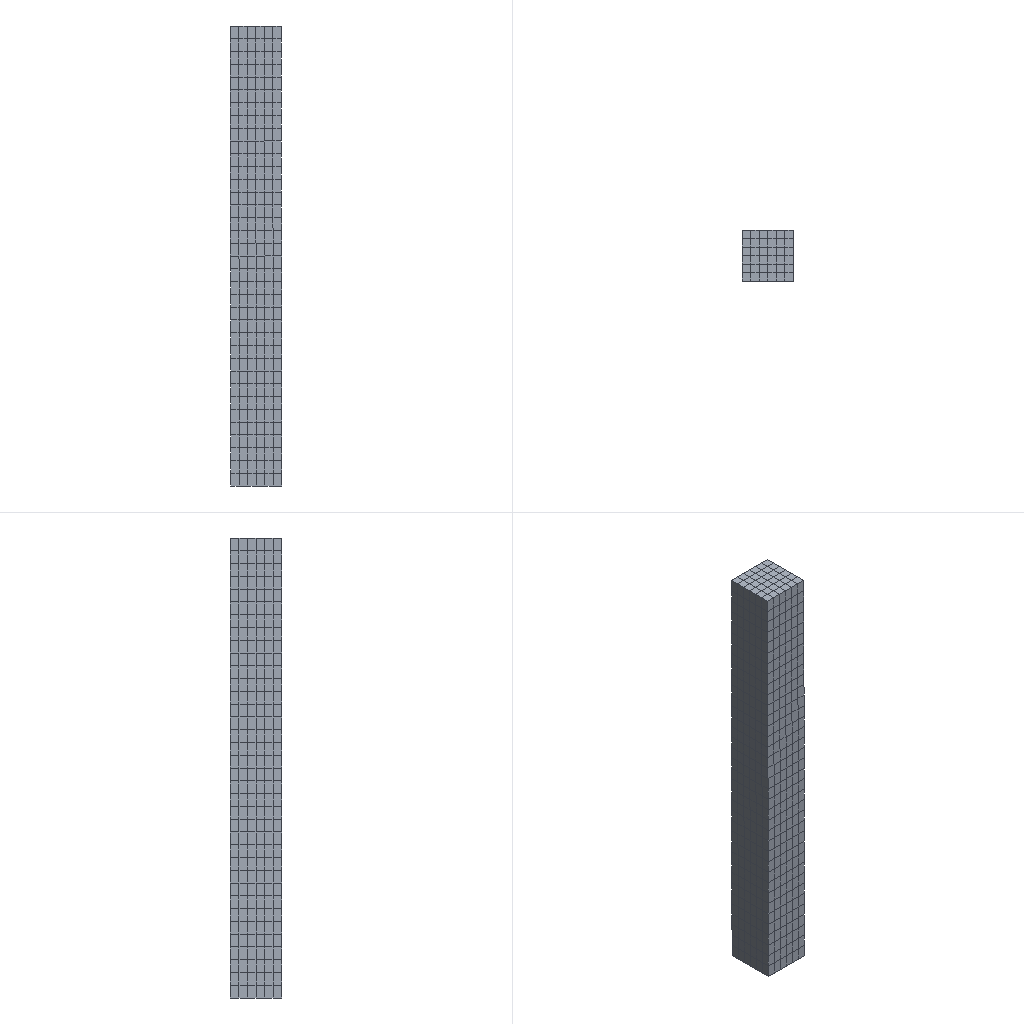Simulation study | abaqus
Set-up summary:
category,name,step,type,value,unit,region
solver,abaqus
solver,version,,,Abaqus/Explicit 2020
units,not stated in the deck,,not stated
analysis,deck,,transient,transient
load_step,Step-1,Step-1,transient,nlgeom=True
contact,interactions,,,general=0 pairs=0 ties=0
load_step,requested,,,1
mesh,nodes,,,2955
mesh,elements,,,2826
element_type,T3D2,,truss,1530
element_type,C3D8R,,solid,1296
load,load commands in deck,,count,1
bc,support commands in deck,,count,7
material,CON,,in results
material,STEEL,,in results
check,setup vs results,,match,"per instance, exact: element labels, types and connectivity; labels of the nodes the elements use; coordinates of those nodes at SINGLE_PRECISION in 1 of 2 instance(s)"
Abaqus input file, long lists of numbers shortened:
*Heading
** Job name: Job-2 Model name: Model-1-Copy
** Generated by: Abaqus/CAE 2020
*Preprint, echo=NO, model=NO, history=NO, contact=NO
**
** PARTS
**
*Part, name=CON-1
*Node
    183, -0.7997,  -400.008,   999.7
    184, -0.7991,  -333.342,   999.701
** (1811 more lines like these left out)
*Element, type=C3D8R
1248, 1749, 1750, 1757, 1756, 1490, 1491, 1498, 1497
1247, 1748, 1749, 1756, 1755, 1489, 1490, 1497, 1496
** (1294 more lines like these left out)
*Nset, nset=SET-1, generate
    1,  1813,     1
*Elset, elset=SET-1, generate
    1,  1296,     1
*Elset, elset=Set-2, generate
    1,  1296,     1
** Section: con
*Solid Section, elset=Set-2, material=con
,
*End Part
**
*Part, name=JIN-FINAL-1
*Node
      1,    374.955,  -375.019,   50.013
      2,   374.951,  -200.,   50.019
** (1140 more lines like these left out)
*Element, type=T3D2
421,  90,  86
361,  86,  83
** (1528 more lines like these left out)
*Nset, nset=SET-1, generate
    1,  1142,     1
*Elset, elset=SET-1, generate
    1,  1530,     1
*Elset, elset=Set-2
    1,    2,    3,    4,    5,    6,    7,    8,   10,   11,   13,   14,   15,   16,   17,   18
   20,   21,   22,   23,   24,   25,   27,   28,   29,   30,   31,   32,   34,   35,   36,   37
** (76 more lines like these left out)
*Elset, elset=Set-3
    9,   12,   19,   26,   33,   40,   46,   50,   54,   64,   65,   69,   73,   77,   81,   88
   95,  102,  109,  120,  126,  135,  139,  145,  146,  149,  153,  154,  155,  159,  169,  170
** (17 more lines like these left out)
*Elset, elset=Set-4
    1,    2,    3,    4,    5,    6,    7,    8,   10,   11,   13,   14,   15,   16,   17,   18
   20,   21,   22,   23,   24,   25,   27,   28,   29,   30,   31,   32,   34,   35,   36,   37
** (76 more lines like these left out)
** Section: zong
*Solid Section, elset=Set-3, material=steel
200.96,
** Section: steel
*Solid Section, elset=Set-4, material=steel
78.5,
*End Part
**
**
** ASSEMBLY
**
*Assembly, name=Assembly
**
*Instance, name=CON-1-1, part=CON-1
*End Instance
**
*Instance, name=JIN-FINAL-1-1, part=JIN-FINAL-1
*End Instance
**
*Node
      1,   195.706,  -200.001,   3599.792
*Nset, nset=Set-5, instance=CON-1-1
  253,  254,  255,  256,  257,  258,  259,  512,  513,  514,  515,  516,  517,  518,  771,  772
  773,  774,  775,  776,  777, 1030, 1031, 1032, 1033, 1034, 1035, 1036, 1289, 1290, 1291, 1292
** (2 more lines like these left out)
*Elset, elset=Set-6, instance=CON-1-1, generate
    1,  1296,     1
*Elset, elset=Set-7, instance=JIN-FINAL-1-1, generate
    1,  1530,     1
*Nset, nset=Set-11
 1,
*Elset, elset=m_Set-8, instance=JIN-FINAL-1-1, generate
    1,  1530,     1
*Nset, nset=m_Set-10
 1,
*Elset, elset=s_Set-8, instance=CON-1-1, generate
    1,  1296,     1
*Elset, elset=_s_Surf-3_S3, internal, instance=CON-1-1
    1,    2,    3,    4,    5,    6,  217,  218,  219,  220,  221,  222,  433,  434,  435,  436
  437,  438,  649,  650,  651,  652,  653,  654,  865,  866,  867,  868,  869,  870, 1081, 1082
** (1 more lines like these left out)
*Surface, type=ELEMENT, name=s_Surf-3
_s_Surf-3_S3, S3
** Constraint: Constraint-1
*Embedded Element, host elset=s_Set-8
m_Set-8
** Constraint: Constraint-2
*Coupling, constraint name=Constraint-2, ref node=m_Set-10, surface=s_Surf-3
*Kinematic
*End Assembly
*Amplitude, name=Amp-1
             0.,              0.,             0.1,              5.,             0.2,              0.,             0.3,             -5.
            0.4,              0.,             0.5,             10.,             0.6,              0.,             0.7,            -10.
            0.8,              0.,             0.9,             20.,              1.,              0.,             1.1,            -20.
            1.2,              0.,             1.3,             35.,             1.4,              0.,             1.5,            -35.
            1.6,              0.,             1.7,             55.,             1.8,              0.,             1.9,            -55.
             2.,              0.,             2.1,             80.,             2.2,              0.,             2.3,            -80.
            2.4,              0.,             2.5,            110.,             2.6,              0.,             2.7,           -110.
            2.8,              0.,             2.9,            145.,              3.,              0.,             3.1,           -145.
            3.2,              0.
**
** MATERIALS
**
*Material, name=con
*Density
 2.5e-09,
*Elastic
32500., 0.2
*Concrete Damaged Plasticity
30.,   0.1,  1.16, 0.667,  0.01
*Concrete Compression Hardening
 31.839,          0.
  35.238, 0.0001688
  37.656, 0.0002734
 39.058, 0.0004092
    39.5, 0.0005746
 38.815, 0.0007747
 37.101,  0.001006
  34.823,  0.001256
 32.332,  0.001511
 29.849,  0.001767
 27.497,  0.002018
 25.334,   0.002263
 23.376,  0.002503
 21.619,  0.002736
 20.051,  0.002963
 18.651,  0.003185
 17.402,  0.003403
 16.285,  0.003616
 15.284,  0.003826
 14.385,   0.004032
 13.573,  0.004236
 12.839,  0.004438
 12.173,  0.004637
 11.567,   0.004835
  11.013,  0.005031
*Concrete Tension Stiffening
  2.09,       0.
   2.4, 8.74e-06
  2.67, 1.23e-05
  2.86, 1.81e-05
  2.94, 2.75e-05
   2.8, 4.37e-05
  2.55, 6.31e-05
   2.3, 8.27e-05
  2.07, 0.000102
  1.86,  0.00012
  1.69, 0.000137
  1.55, 0.000153
  1.42, 0.000169
  1.31, 0.000184
  1.22, 0.000198
  1.14, 0.000213
  1.07, 0.000227
  1.01,  0.00024
 0.956, 0.000254
 0.908, 0.000267
 0.864,  0.00028
 0.825, 0.000293
 0.789, 0.000306
 0.757, 0.000319
 0.727, 0.000332
*Concrete Compression Damage
        0.,          0.
 0.06977, 0.0001688
  0.1005, 0.0002734
  0.1363, 0.0004092
  0.176, 0.0005746
  0.2212, 0.0007747
  0.271,  0.001006
  0.3214,  0.001256
  0.3699,  0.001511
  0.4151,  0.001767
  0.4565,  0.002018
  0.4939,   0.002263
  0.5275,  0.002503
   0.5577,  0.002736
  0.5849,  0.002963
   0.6093,  0.003185
  0.6313,  0.003403
  0.6511,  0.003616
  0.6691,  0.003826
  0.6855,   0.004032
  0.7004,  0.004236
  0.7141,  0.004438
  0.7266,  0.004637
  0.7382,   0.004835
  0.7488,  0.005031
  0.7586,  0.005226
  0.7678,  0.005419
  0.7763,  0.005611
  0.7842,  0.005802
  0.7915,  0.005993
  0.7984,  0.006182
  0.8049,  0.006371
  0.811,  0.006559
  0.8167,  0.006747
  0.8221,  0.006933
  0.8627,  0.008781
  0.8884,   0.01061
  0.906,   0.01242
  0.9188,   0.01423
  0.9286,   0.01603
** (21 more lines like these left out)
*Concrete Tension Damage, compression recovery=0.45
     0.,       0.
 0.0544, 8.74e-06
 0.0674, 1.23e-05
 0.0893, 1.81e-05
  0.124, 2.75e-05
  0.186, 4.37e-05
  0.255, 6.31e-05
  0.321, 8.27e-05
   0.38, 0.000102
  0.431,  0.00012
  0.475, 0.000137
  0.513, 0.000153
  0.546, 0.000169
  0.575, 0.000184
  0.601, 0.000198
  0.623, 0.000213
  0.643, 0.000227
  0.661,  0.00024
  0.678, 0.000254
  0.692, 0.000267
  0.706,  0.00028
  0.718, 0.000293
  0.729, 0.000306
  0.739, 0.000319
  0.749, 0.000332
  0.757, 0.000344
  0.765, 0.000357
  0.773, 0.000369
   0.78, 0.000382
  0.787, 0.000394
  0.793, 0.000407
  0.799, 0.000419
  0.804, 0.000431
  0.809, 0.000443
  0.814, 0.000456
  0.851, 0.000577
  0.875, 0.000697
  0.892, 0.000816
  0.905, 0.000935
  0.915,  0.00105
** (31 more lines like these left out)
*Material, name=steel
*Density
 7.8e-09,
*Elastic
210000., 0.3
*Plastic
247.,0.
**
** PREDEFINED FIELDS
**
** Name: Predefined Field-1   Type: Stress
*Initial Conditions, type=STRESS, file=D:/TNTandZhihui/model/Job-1.odb, step=1, inc=1785
** Name: Predefined Field-2   Type: Stress
*Initial Conditions, type=STRESS, file=D:/TNTandZhihui/model/Job-1.odb, step=1, inc=1785
** ----------------------------------------------------------------
**
** STEP: Step-1
**
*Step, name=Step-1, nlgeom=YES
*Dynamic, Explicit
, 3.2
*Bulk Viscosity
0.06, 1.2
**
** BOUNDARY CONDITIONS
**
** Name: BC-1 Type: 对称/反对称/完全固定
*Boundary
Set-5, ENCASTRE
** Name: [REDACTED] : Displacement/rotation angle
*Boundary, amplitude=Amp-1
Set-11, 1, 1, 1.
Set-11, 2, 2
Set-11, 3, 3
Set-11, 4, 4
Set-11, 5, 5
Set-11, 6, 6
**
** OUTPUT REQUESTS
**
*Restart, write, number interval=1, time marks=NO
**
** FIELD OUTPUT: F-Output-1
**
*Output, field, number interval=100
*Node Output
CF, RF, RM, RT, U, V
*Element Output, directions=YES
DAMAGEC, DAMAGET, E, LE, MISES, MISESMAX, MISESONLY, NE, PE, PEEQ, PEEQMAX, PEEQT, PEMAG, PRESSONLY, S, SDEG
SEQUT, SF, SSAVG, YIELDPOT
*Contact Output
CDISP, CFORCE, CSTRESS, PPRESS
**
** HISTORY OUTPUT: H-Output-1
**
*Output, history, time interval=3.2e-05
*Node Output, nset=Set-11
RF1, U1
*End Step
Results summary:
result,step,Step-1,completed,increments=597134 time=3.2/3.2
result,analysis,,,transient
result,last_loadstep,,,1
result,analysis steps,,count,1
result,primary field,,,U
result,reaction total,,FX,-96234.916,model units
result,reaction total,,FY,-10890.557,model units
result,reaction total,,FZ,1923.785,model units